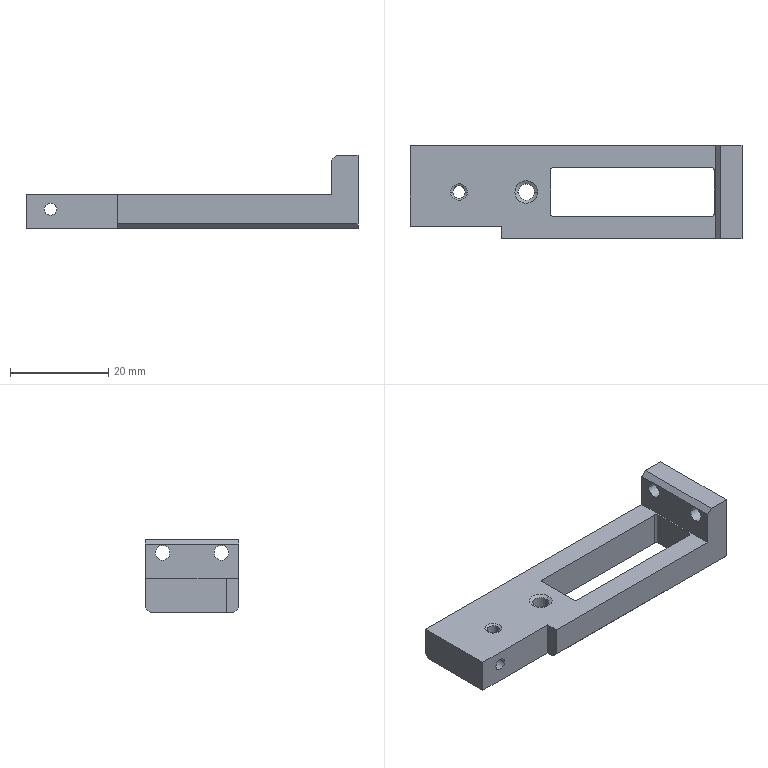Part | NX | 1 solid | 40 faces | box 67.7 x 19 x 15 mm | volume 6801 mm3 | plane 18 | cylinder 16 | cone 6 | commonest cylinder face diameters 1 x4 2.5 x4 3 x4 3.3 x2 4 x2
STEP:
#1=CARTESIAN_POINT('',(-33.85,-7.,3.5));
#2=VERTEX_POINT('',#1);
#3=CARTESIAN_POINT('',(-33.85,-7.,-3.5));
#4=VERTEX_POINT('',#3);
#5=CARTESIAN_POINT('',(-33.85,-7.,0.));
#6=DIRECTION('',(0.,0.,-1.));
#7=VECTOR('',#6,1000.);
#8=LINE('',#5,#7);
#9=EDGE_CURVE('',#2,#4,#8,.T.);
#10=ORIENTED_EDGE('',*,*,#9,.F.);
#11=CARTESIAN_POINT('',(-33.85,9.5,3.5));
#12=VERTEX_POINT('',#11);
#13=CARTESIAN_POINT('',(-33.85,0.,3.5));
#14=DIRECTION('',(0.,1.,0.));
#15=VECTOR('',#14,1000.);
#16=LINE('',#13,#15);
#17=EDGE_CURVE('',#2,#12,#16,.T.);
#18=ORIENTED_EDGE('',*,*,#17,.T.);
#19=CARTESIAN_POINT('',(-33.85,9.5,-2.5));
#20=VERTEX_POINT('',#19);
#21=CARTESIAN_POINT('',(-33.85,9.5,0.));
#22=DIRECTION('',(0.,0.,-1.));
#23=VECTOR('',#22,1000.);
#24=LINE('',#21,#23);
#25=EDGE_CURVE('',#12,#20,#24,.T.);
#26=ORIENTED_EDGE('',*,*,#25,.T.);
#27=CARTESIAN_POINT('',(-33.85,8.5,-3.5));
#28=VERTEX_POINT('',#27);
#29=CARTESIAN_POINT('',(-33.85,12.,0.));
#30=DIRECTION('',(0.,0.7071,0.7071));
#31=VECTOR('',#30,1000.);
#32=LINE('',#29,#31);
#33=EDGE_CURVE('',#28,#20,#32,.T.);
#34=ORIENTED_EDGE('',*,*,#33,.F.);
#35=CARTESIAN_POINT('',(-33.85,0.,-3.5));
#36=DIRECTION('',(0.,1.,0.));
#37=VECTOR('',#36,1000.);
#38=LINE('',#35,#37);
#39=EDGE_CURVE('',#4,#28,#38,.T.);
#40=ORIENTED_EDGE('',*,*,#39,.F.);
#41=EDGE_LOOP('',(#10,#18,#26,#34,#40));
#42=FACE_BOUND('',#41,.T.);
#43=CARTESIAN_POINT('',(-33.85,9.5,-3.5));
#44=DIRECTION('',(-1.,0.,0.));
#45=DIRECTION('',(0.,0.,1.));
#46=AXIS2_PLACEMENT_3D('',#43,#44,#45);
#47=PLANE('',#46);
#48=ADVANCED_FACE('',(#42),#47,.T.);
#49=CARTESIAN_POINT('',(-15.15,-7.,-3.5));
#50=VERTEX_POINT('',#49);
#51=CARTESIAN_POINT('',(-15.15,-8.5,-3.5));
#52=VERTEX_POINT('',#51);
#53=CARTESIAN_POINT('',(-15.15,0.,-3.5));
#54=DIRECTION('',(0.,-1.,0.));
#55=VECTOR('',#54,1000.);
#56=LINE('',#53,#55);
#57=EDGE_CURVE('',#50,#52,#56,.T.);
#58=ORIENTED_EDGE('',*,*,#57,.T.);
#59=CARTESIAN_POINT('',(-15.15,-9.5,-2.5));
#60=VERTEX_POINT('',#59);
#61=CARTESIAN_POINT('',(-15.15,-9.5,-2.5));
#62=DIRECTION('',(0.,0.7071,-0.7071));
#63=VECTOR('',#62,1000.);
#64=LINE('',#61,#63);
#65=EDGE_CURVE('',#60,#52,#64,.T.);
#66=ORIENTED_EDGE('',*,*,#65,.F.);
#67=CARTESIAN_POINT('',(-15.15,-9.5,3.5));
#68=VERTEX_POINT('',#67);
#69=CARTESIAN_POINT('',(-15.15,-9.5,3.5));
#70=DIRECTION('',(0.,0.,-1.));
#71=VECTOR('',#70,1000.);
#72=LINE('',#69,#71);
#73=EDGE_CURVE('',#68,#60,#72,.T.);
#74=ORIENTED_EDGE('',*,*,#73,.F.);
#75=CARTESIAN_POINT('',(-15.15,-7.,3.5));
#76=VERTEX_POINT('',#75);
#77=CARTESIAN_POINT('',(-15.15,0.,3.5));
#78=DIRECTION('',(0.,-1.,0.));
#79=VECTOR('',#78,1000.);
#80=LINE('',#77,#79);
#81=EDGE_CURVE('',#76,#68,#80,.T.);
#82=ORIENTED_EDGE('',*,*,#81,.F.);
#83=CARTESIAN_POINT('',(-15.15,-7.,0.));
#84=DIRECTION('',(0.,0.,1.));
#85=VECTOR('',#84,1000.);
#86=LINE('',#83,#85);
#87=EDGE_CURVE('',#50,#76,#86,.T.);
#88=ORIENTED_EDGE('',*,*,#87,.F.);
#89=EDGE_LOOP('',(#58,#66,#74,#82,#88));
#90=FACE_BOUND('',#89,.T.);
#91=CARTESIAN_POINT('',(-15.15,-9.5,3.5));
#92=DIRECTION('',(1.,0.,0.));
#93=DIRECTION('',(0.,1.,0.));
#94=AXIS2_PLACEMENT_3D('',#91,#92,#93);
#95=PLANE('',#94);
#96=ADVANCED_FACE('',(#90),#95,.F.);
#97=ORIENTED_EDGE('',*,*,#81,.T.);
#98=CARTESIAN_POINT('',(28.5,-9.5,3.5));
#99=VERTEX_POINT('',#98);
#100=CARTESIAN_POINT('',(0.,-9.5,3.5));
#101=DIRECTION('',(-1.,0.,0.));
#102=VECTOR('',#101,1000.);
#103=LINE('',#100,#102);
#104=EDGE_CURVE('',#99,#68,#103,.T.);
#105=ORIENTED_EDGE('',*,*,#104,.F.);
#106=CARTESIAN_POINT('',(28.5,9.5,3.5));
#107=VERTEX_POINT('',#106);
#108=CARTESIAN_POINT('',(28.5,0.,3.5));
#109=DIRECTION('',(0.,1.,0.));
#110=VECTOR('',#109,1000.);
#111=LINE('',#108,#110);
#112=EDGE_CURVE('',#99,#107,#111,.T.);
#113=ORIENTED_EDGE('',*,*,#112,.T.);
#114=CARTESIAN_POINT('',(0.,9.5,3.5));
#115=DIRECTION('',(1.,0.,0.));
#116=VECTOR('',#115,1000.);
#117=LINE('',#114,#116);
#118=EDGE_CURVE('',#12,#107,#117,.T.);
#119=ORIENTED_EDGE('',*,*,#118,.F.);
#120=ORIENTED_EDGE('',*,*,#17,.F.);
#121=CARTESIAN_POINT('',(0.,-7.,3.5));
#122=DIRECTION('',(1.,0.,0.));
#123=VECTOR('',#122,1000.);
#124=LINE('',#121,#123);
#125=EDGE_CURVE('',#2,#76,#124,.T.);
#126=ORIENTED_EDGE('',*,*,#125,.T.);
#127=EDGE_LOOP('',(#97,#105,#113,#119,#120,#126));
#128=FACE_BOUND('',#127,.T.);
#129=CARTESIAN_POINT('',(27.65,-5.,3.5));
#130=VERTEX_POINT('',#129);
#131=CARTESIAN_POINT('',(-4.65,-5.,3.5));
#132=VERTEX_POINT('',#131);
#133=CARTESIAN_POINT('',(0.,-5.,3.5));
#134=DIRECTION('',(-1.,0.,0.));
#135=VECTOR('',#134,1000.);
#136=LINE('',#133,#135);
#137=EDGE_CURVE('',#130,#132,#136,.T.);
#138=ORIENTED_EDGE('',*,*,#137,.T.);
#139=CARTESIAN_POINT('',(-5.15,-4.5,3.5));
#140=VERTEX_POINT('',#139);
#141=CARTESIAN_POINT('',(-4.65,-4.5,3.5));
#142=DIRECTION('',(0.,0.,1.));
#143=DIRECTION('',(0.,1.,0.));
#144=AXIS2_PLACEMENT_3D('',#141,#142,#143);
#145=CIRCLE('',#144,0.5);
#146=EDGE_CURVE('',#140,#132,#145,.T.);
#147=ORIENTED_EDGE('',*,*,#146,.F.);
#148=CARTESIAN_POINT('',(-5.15,4.5,3.5));
#149=VERTEX_POINT('',#148);
#150=CARTESIAN_POINT('',(-5.15,0.,3.5));
#151=DIRECTION('',(0.,1.,0.));
#152=VECTOR('',#151,1000.);
#153=LINE('',#150,#152);
#154=EDGE_CURVE('',#140,#149,#153,.T.);
#155=ORIENTED_EDGE('',*,*,#154,.T.);
#156=CARTESIAN_POINT('',(-4.65,5.,3.5));
#157=VERTEX_POINT('',#156);
#158=CARTESIAN_POINT('',(-4.65,4.5,3.5));
#159=DIRECTION('',(0.,0.,1.));
#160=DIRECTION('',(0.,1.,0.));
#161=AXIS2_PLACEMENT_3D('',#158,#159,#160);
#162=CIRCLE('',#161,0.5);
#163=EDGE_CURVE('',#157,#149,#162,.T.);
#164=ORIENTED_EDGE('',*,*,#163,.F.);
#165=CARTESIAN_POINT('',(27.65,5.,3.5));
#166=VERTEX_POINT('',#165);
#167=CARTESIAN_POINT('',(0.,5.,3.5));
#168=DIRECTION('',(1.,0.,0.));
#169=VECTOR('',#168,1000.);
#170=LINE('',#167,#169);
#171=EDGE_CURVE('',#157,#166,#170,.T.);
#172=ORIENTED_EDGE('',*,*,#171,.T.);
#173=CARTESIAN_POINT('',(28.15,4.5,3.5));
#174=VERTEX_POINT('',#173);
#175=CARTESIAN_POINT('',(27.65,4.5,3.5));
#176=DIRECTION('',(0.,0.,1.));
#177=DIRECTION('',(0.,1.,0.));
#178=AXIS2_PLACEMENT_3D('',#175,#176,#177);
#179=CIRCLE('',#178,0.5);
#180=EDGE_CURVE('',#174,#166,#179,.T.);
#181=ORIENTED_EDGE('',*,*,#180,.F.);
#182=CARTESIAN_POINT('',(28.15,-4.5,3.5));
#183=VERTEX_POINT('',#182);
#184=CARTESIAN_POINT('',(28.15,0.,3.5));
#185=DIRECTION('',(0.,-1.,0.));
#186=VECTOR('',#185,1000.);
#187=LINE('',#184,#186);
#188=EDGE_CURVE('',#174,#183,#187,.T.);
#189=ORIENTED_EDGE('',*,*,#188,.T.);
#190=CARTESIAN_POINT('',(27.65,-4.5,3.5));
#191=DIRECTION('',(0.,0.,1.));
#192=DIRECTION('',(0.,1.,0.));
#193=AXIS2_PLACEMENT_3D('',#190,#191,#192);
#194=CIRCLE('',#193,0.5);
#195=EDGE_CURVE('',#130,#183,#194,.T.);
#196=ORIENTED_EDGE('',*,*,#195,.F.);
#197=EDGE_LOOP('',(#138,#147,#155,#164,#172,#181,#189,#196));
#198=FACE_BOUND('',#197,.T.);
#199=CARTESIAN_POINT('',(-12.465,0.,3.5));
#200=VERTEX_POINT('',#199);
#201=CARTESIAN_POINT('',(-7.835,0.,3.5));
#202=VERTEX_POINT('',#201);
#203=CARTESIAN_POINT('',(-10.15,0.,3.5));
#204=DIRECTION('',(0.,0.,1.));
#205=DIRECTION('',(1.,0.,0.));
#206=AXIS2_PLACEMENT_3D('',#203,#204,#205);
#207=CIRCLE('',#206,2.315);
#208=EDGE_CURVE('',#200,#202,#207,.T.);
#209=ORIENTED_EDGE('',*,*,#208,.F.);
#210=CARTESIAN_POINT('',(-10.15,0.,3.5));
#211=DIRECTION('',(0.,0.,1.));
#212=DIRECTION('',(1.,0.,0.));
#213=AXIS2_PLACEMENT_3D('',#210,#211,#212);
#214=CIRCLE('',#213,2.315);
#215=EDGE_CURVE('',#202,#200,#214,.T.);
#216=ORIENTED_EDGE('',*,*,#215,.F.);
#217=EDGE_LOOP('',(#209,#216));
#218=FACE_BOUND('',#217,.T.);
#219=CARTESIAN_POINT('',(-25.55,0.,3.5));
#220=VERTEX_POINT('',#219);
#221=CARTESIAN_POINT('',(-22.15,0.,3.5));
#222=VERTEX_POINT('',#221);
#223=CARTESIAN_POINT('',(-23.85,0.,3.5));
#224=DIRECTION('',(0.,0.,1.));
#225=DIRECTION('',(1.,0.,0.));
#226=AXIS2_PLACEMENT_3D('',#223,#224,#225);
#227=CIRCLE('',#226,1.7);
#228=EDGE_CURVE('',#220,#222,#227,.T.);
#229=ORIENTED_EDGE('',*,*,#228,.F.);
#230=CARTESIAN_POINT('',(-23.85,0.,3.5));
#231=DIRECTION('',(0.,0.,1.));
#232=DIRECTION('',(1.,0.,0.));
#233=AXIS2_PLACEMENT_3D('',#230,#231,#232);
#234=CIRCLE('',#233,1.7);
#235=EDGE_CURVE('',#222,#220,#234,.T.);
#236=ORIENTED_EDGE('',*,*,#235,.F.);
#237=EDGE_LOOP('',(#229,#236));
#238=FACE_BOUND('',#237,.T.);
#239=CARTESIAN_POINT('',(0.,0.,3.5));
#240=DIRECTION('',(0.,0.,1.));
#241=DIRECTION('',(1.,0.,0.));
#242=AXIS2_PLACEMENT_3D('',#239,#240,#241);
#243=PLANE('',#242);
#244=ADVANCED_FACE('',(#128,#198,#218,#238),#243,.T.);
#245=ORIENTED_EDGE('',*,*,#112,.F.);
#246=CARTESIAN_POINT('',(28.5,-9.5,10.5));
#247=VERTEX_POINT('',#246);
#248=CARTESIAN_POINT('',(28.5,-9.5,0.));
#249=DIRECTION('',(0.,0.,-1.));
#250=VECTOR('',#249,1000.);
#251=LINE('',#248,#250);
#252=EDGE_CURVE('',#247,#99,#251,.T.);
#253=ORIENTED_EDGE('',*,*,#252,.F.);
#254=CARTESIAN_POINT('',(28.5,9.5,10.5));
#255=VERTEX_POINT('',#254);
#256=CARTESIAN_POINT('',(28.5,0.,10.5));
#257=DIRECTION('',(0.,1.,0.));
#258=VECTOR('',#257,1000.);
#259=LINE('',#256,#258);
#260=EDGE_CURVE('',#247,#255,#259,.T.);
#261=ORIENTED_EDGE('',*,*,#260,.T.);
#262=CARTESIAN_POINT('',(28.5,9.5,0.));
#263=DIRECTION('',(0.,0.,-1.));
#264=VECTOR('',#263,1000.);
#265=LINE('',#262,#264);
#266=EDGE_CURVE('',#255,#107,#265,.T.);
#267=ORIENTED_EDGE('',*,*,#266,.T.);
#268=EDGE_LOOP('',(#245,#253,#261,#267));
#269=FACE_BOUND('',#268,.T.);
#270=CARTESIAN_POINT('',(28.5,-7.5,8.73));
#271=VERTEX_POINT('',#270);
#272=CARTESIAN_POINT('',(28.5,-4.5,8.73));
#273=VERTEX_POINT('',#272);
#274=CARTESIAN_POINT('',(28.5,-6.,8.73));
#275=DIRECTION('',(1.,0.,0.));
#276=DIRECTION('',(0.,1.,0.));
#277=AXIS2_PLACEMENT_3D('',#274,#275,#276);
#278=CIRCLE('',#277,1.5);
#279=EDGE_CURVE('',#271,#273,#278,.T.);
#280=ORIENTED_EDGE('',*,*,#279,.T.);
#281=CARTESIAN_POINT('',(28.5,-6.,8.73));
#282=DIRECTION('',(1.,0.,0.));
#283=DIRECTION('',(0.,1.,0.));
#284=AXIS2_PLACEMENT_3D('',#281,#282,#283);
#285=CIRCLE('',#284,1.5);
#286=EDGE_CURVE('',#273,#271,#285,.T.);
#287=ORIENTED_EDGE('',*,*,#286,.T.);
#288=EDGE_LOOP('',(#280,#287));
#289=FACE_BOUND('',#288,.T.);
#290=CARTESIAN_POINT('',(28.5,7.5,8.73));
#291=VERTEX_POINT('',#290);
#292=CARTESIAN_POINT('',(28.5,4.5,8.73));
#293=VERTEX_POINT('',#292);
#294=CARTESIAN_POINT('',(28.5,6.,8.73));
#295=DIRECTION('',(1.,0.,0.));
#296=DIRECTION('',(0.,1.,0.));
#297=AXIS2_PLACEMENT_3D('',#294,#295,#296);
#298=CIRCLE('',#297,1.5);
#299=EDGE_CURVE('',#291,#293,#298,.T.);
#300=ORIENTED_EDGE('',*,*,#299,.T.);
#301=CARTESIAN_POINT('',(28.5,6.,8.73));
#302=DIRECTION('',(1.,0.,0.));
#303=DIRECTION('',(0.,1.,0.));
#304=AXIS2_PLACEMENT_3D('',#301,#302,#303);
#305=CIRCLE('',#304,1.5);
#306=EDGE_CURVE('',#293,#291,#305,.T.);
#307=ORIENTED_EDGE('',*,*,#306,.T.);
#308=EDGE_LOOP('',(#300,#307));
#309=FACE_BOUND('',#308,.T.);
#310=CARTESIAN_POINT('',(28.5,9.5,3.5));
#311=DIRECTION('',(-1.,0.,0.));
#312=DIRECTION('',(0.,0.,1.));
#313=AXIS2_PLACEMENT_3D('',#310,#311,#312);
#314=PLANE('',#313);
#315=ADVANCED_FACE('',(#269,#289,#309),#314,.T.);
#316=CARTESIAN_POINT('',(33.85,9.5,-2.5));
#317=VERTEX_POINT('',#316);
#318=CARTESIAN_POINT('',(0.,9.5,-2.5));
#319=DIRECTION('',(1.,0.,0.));
#320=VECTOR('',#319,1000.);
#321=LINE('',#318,#320);
#322=EDGE_CURVE('',#20,#317,#321,.T.);
#323=ORIENTED_EDGE('',*,*,#322,.F.);
#324=ORIENTED_EDGE('',*,*,#25,.F.);
#325=ORIENTED_EDGE('',*,*,#118,.T.);
#326=ORIENTED_EDGE('',*,*,#266,.F.);
#327=CARTESIAN_POINT('',(29.5,9.5,11.5));
#328=VERTEX_POINT('',#327);
#329=CARTESIAN_POINT('',(18.,9.5,0.));
#330=DIRECTION('',(0.7071,0.,0.7071));
#331=VECTOR('',#330,1000.);
#332=LINE('',#329,#331);
#333=EDGE_CURVE('',#255,#328,#332,.T.);
#334=ORIENTED_EDGE('',*,*,#333,.T.);
#335=CARTESIAN_POINT('',(33.85,9.5,11.5));
#336=VERTEX_POINT('',#335);
#337=CARTESIAN_POINT('',(0.,9.5,11.5));
#338=DIRECTION('',(-1.,0.,0.));
#339=VECTOR('',#338,1000.);
#340=LINE('',#337,#339);
#341=EDGE_CURVE('',#336,#328,#340,.T.);
#342=ORIENTED_EDGE('',*,*,#341,.F.);
#343=CARTESIAN_POINT('',(33.85,9.5,0.));
#344=DIRECTION('',(0.,0.,1.));
#345=VECTOR('',#344,1000.);
#346=LINE('',#343,#345);
#347=EDGE_CURVE('',#317,#336,#346,.T.);
#348=ORIENTED_EDGE('',*,*,#347,.F.);
#349=EDGE_LOOP('',(#323,#324,#325,#326,#334,#342,#348));
#350=FACE_BOUND('',#349,.T.);
#351=CARTESIAN_POINT('',(-30.85,9.5,0.5));
#352=VERTEX_POINT('',#351);
#353=CARTESIAN_POINT('',(-26.85,9.5,0.5));
#354=VERTEX_POINT('',#353);
#355=CARTESIAN_POINT('',(-28.85,9.5,0.5));
#356=DIRECTION('',(0.,1.,0.));
#357=DIRECTION('',(-1.,0.,0.));
#358=AXIS2_PLACEMENT_3D('',#355,#356,#357);
#359=CIRCLE('',#358,2.);
#360=EDGE_CURVE('',#352,#354,#359,.T.);
#361=ORIENTED_EDGE('',*,*,#360,.F.);
#362=CARTESIAN_POINT('',(-28.85,9.5,0.5));
#363=DIRECTION('',(0.,1.,0.));
#364=DIRECTION('',(-1.,0.,0.));
#365=AXIS2_PLACEMENT_3D('',#362,#363,#364);
#366=CIRCLE('',#365,2.);
#367=EDGE_CURVE('',#354,#352,#366,.T.);
#368=ORIENTED_EDGE('',*,*,#367,.F.);
#369=EDGE_LOOP('',(#361,#368));
#370=FACE_BOUND('',#369,.T.);
#371=CARTESIAN_POINT('',(33.85,9.5,-3.5));
#372=DIRECTION('',(0.,1.,0.));
#373=DIRECTION('',(1.,0.,0.));
#374=AXIS2_PLACEMENT_3D('',#371,#372,#373);
#375=PLANE('',#374);
#376=ADVANCED_FACE('',(#350,#370),#375,.T.);
#377=ORIENTED_EDGE('',*,*,#228,.T.);
#378=CARTESIAN_POINT('',(-22.6,0.,3.24));
#379=VERTEX_POINT('',#378);
#380=CARTESIAN_POINT('',(-22.6,0.,3.24));
#381=DIRECTION('',(0.866,0.,0.5));
#382=VECTOR('',#381,1000.);
#383=LINE('',#380,#382);
#384=EDGE_CURVE('',#379,#222,#383,.T.);
#385=ORIENTED_EDGE('',*,*,#384,.F.);
#386=CARTESIAN_POINT('',(-25.1,0.,3.24));
#387=VERTEX_POINT('',#386);
#388=CARTESIAN_POINT('',(-23.85,0.,3.24));
#389=DIRECTION('',(0.,0.,1.));
#390=DIRECTION('',(1.,0.,0.));
#391=AXIS2_PLACEMENT_3D('',#388,#389,#390);
#392=CIRCLE('',#391,1.25);
#393=EDGE_CURVE('',#387,#379,#392,.T.);
#394=ORIENTED_EDGE('',*,*,#393,.F.);
#395=CARTESIAN_POINT('',(-25.1,0.,3.24));
#396=DIRECTION('',(-0.866,0.,0.5));
#397=VECTOR('',#396,1000.);
#398=LINE('',#395,#397);
#399=EDGE_CURVE('',#387,#220,#398,.T.);
#400=ORIENTED_EDGE('',*,*,#399,.T.);
#401=EDGE_LOOP('',(#377,#385,#394,#400));
#402=FACE_BOUND('',#401,.T.);
#403=CARTESIAN_POINT('',(-23.85,0.,3.24));
#404=DIRECTION('',(0.,0.,1.));
#405=DIRECTION('',(1.,0.,0.));
#406=AXIS2_PLACEMENT_3D('',#403,#404,#405);
#407=CONICAL_SURFACE('',#406,1.25,1.047);
#408=ADVANCED_FACE('',(#402),#407,.F.);
#409=CARTESIAN_POINT('',(-25.1,0.,-3.5));
#410=VERTEX_POINT('',#409);
#411=CARTESIAN_POINT('',(-22.6,0.,-3.5));
#412=VERTEX_POINT('',#411);
#413=CARTESIAN_POINT('',(-23.85,0.,-3.5));
#414=DIRECTION('',(0.,0.,1.));
#415=DIRECTION('',(1.,0.,0.));
#416=AXIS2_PLACEMENT_3D('',#413,#414,#415);
#417=CIRCLE('',#416,1.25);
#418=EDGE_CURVE('',#410,#412,#417,.T.);
#419=ORIENTED_EDGE('',*,*,#418,.F.);
#420=CARTESIAN_POINT('',(-25.1,0.,3.5));
#421=DIRECTION('',(0.,0.,1.));
#422=VECTOR('',#421,1000.);
#423=LINE('',#420,#422);
#424=EDGE_CURVE('',#410,#387,#423,.T.);
#425=ORIENTED_EDGE('',*,*,#424,.T.);
#426=ORIENTED_EDGE('',*,*,#393,.T.);
#427=CARTESIAN_POINT('',(-22.6,0.,3.5));
#428=DIRECTION('',(0.,0.,1.));
#429=VECTOR('',#428,1000.);
#430=LINE('',#427,#429);
#431=EDGE_CURVE('',#412,#379,#430,.T.);
#432=ORIENTED_EDGE('',*,*,#431,.F.);
#433=EDGE_LOOP('',(#419,#425,#426,#432));
#434=FACE_BOUND('',#433,.T.);
#435=CARTESIAN_POINT('',(-23.85,0.,3.5));
#436=DIRECTION('',(0.,0.,1.));
#437=DIRECTION('',(1.,0.,0.));
#438=AXIS2_PLACEMENT_3D('',#435,#436,#437);
#439=CYLINDRICAL_SURFACE('',#438,1.25);
#440=ADVANCED_FACE('',(#434),#439,.F.);
#441=ORIENTED_EDGE('',*,*,#347,.T.);
#442=CARTESIAN_POINT('',(33.85,-9.5,11.5));
#443=VERTEX_POINT('',#442);
#444=CARTESIAN_POINT('',(33.85,0.,11.5));
#445=DIRECTION('',(0.,1.,0.));
#446=VECTOR('',#445,1000.);
#447=LINE('',#444,#446);
#448=EDGE_CURVE('',#443,#336,#447,.T.);
#449=ORIENTED_EDGE('',*,*,#448,.F.);
#450=CARTESIAN_POINT('',(33.85,-9.5,-2.5));
#451=VERTEX_POINT('',#450);
#452=CARTESIAN_POINT('',(33.85,-9.5,0.));
#453=DIRECTION('',(0.,0.,1.));
#454=VECTOR('',#453,1000.);
#455=LINE('',#452,#454);
#456=EDGE_CURVE('',#451,#443,#455,.T.);
#457=ORIENTED_EDGE('',*,*,#456,.F.);
#458=CARTESIAN_POINT('',(33.85,-8.5,-3.5));
#459=VERTEX_POINT('',#458);
#460=CARTESIAN_POINT('',(33.85,-12.,0.));
#461=DIRECTION('',(0.,-0.7071,0.7071));
#462=VECTOR('',#461,1000.);
#463=LINE('',#460,#462);
#464=EDGE_CURVE('',#459,#451,#463,.T.);
#465=ORIENTED_EDGE('',*,*,#464,.F.);
#466=CARTESIAN_POINT('',(33.85,8.5,-3.5));
#467=VERTEX_POINT('',#466);
#468=CARTESIAN_POINT('',(33.85,0.,-3.5));
#469=DIRECTION('',(0.,-1.,0.));
#470=VECTOR('',#469,1000.);
#471=LINE('',#468,#470);
#472=EDGE_CURVE('',#467,#459,#471,.T.);
#473=ORIENTED_EDGE('',*,*,#472,.F.);
#474=CARTESIAN_POINT('',(33.85,12.,0.));
#475=DIRECTION('',(0.,-0.7071,-0.7071));
#476=VECTOR('',#475,1000.);
#477=LINE('',#474,#476);
#478=EDGE_CURVE('',#317,#467,#477,.T.);
#479=ORIENTED_EDGE('',*,*,#478,.F.);
#480=EDGE_LOOP('',(#441,#449,#457,#465,#473,#479));
#481=FACE_BOUND('',#480,.T.);
#482=CARTESIAN_POINT('',(33.85,-4.5,8.73));
#483=VERTEX_POINT('',#482);
#484=CARTESIAN_POINT('',(33.85,-7.5,8.73));
#485=VERTEX_POINT('',#484);
#486=CARTESIAN_POINT('',(33.85,-6.,8.73));
#487=DIRECTION('',(1.,0.,0.));
#488=DIRECTION('',(0.,1.,0.));
#489=AXIS2_PLACEMENT_3D('',#486,#487,#488);
#490=CIRCLE('',#489,1.5);
#491=EDGE_CURVE('',#483,#485,#490,.T.);
#492=ORIENTED_EDGE('',*,*,#491,.F.);
#493=CARTESIAN_POINT('',(33.85,-6.,8.73));
#494=DIRECTION('',(1.,0.,0.));
#495=DIRECTION('',(0.,1.,0.));
#496=AXIS2_PLACEMENT_3D('',#493,#494,#495);
#497=CIRCLE('',#496,1.5);
#498=EDGE_CURVE('',#485,#483,#497,.T.);
#499=ORIENTED_EDGE('',*,*,#498,.F.);
#500=EDGE_LOOP('',(#492,#499));
#501=FACE_BOUND('',#500,.T.);
#502=CARTESIAN_POINT('',(33.85,7.5,8.73));
#503=VERTEX_POINT('',#502);
#504=CARTESIAN_POINT('',(33.85,4.5,8.73));
#505=VERTEX_POINT('',#504);
#506=CARTESIAN_POINT('',(33.85,6.,8.73));
#507=DIRECTION('',(1.,0.,0.));
#508=DIRECTION('',(0.,1.,0.));
#509=AXIS2_PLACEMENT_3D('',#506,#507,#508);
#510=CIRCLE('',#509,1.5);
#511=EDGE_CURVE('',#503,#505,#510,.T.);
#512=ORIENTED_EDGE('',*,*,#511,.F.);
#513=CARTESIAN_POINT('',(33.85,6.,8.73));
#514=DIRECTION('',(1.,0.,0.));
#515=DIRECTION('',(0.,1.,0.));
#516=AXIS2_PLACEMENT_3D('',#513,#514,#515);
#517=CIRCLE('',#516,1.5);
#518=EDGE_CURVE('',#505,#503,#517,.T.);
#519=ORIENTED_EDGE('',*,*,#518,.F.);
#520=EDGE_LOOP('',(#512,#519));
#521=FACE_BOUND('',#520,.T.);
#522=CARTESIAN_POINT('',(33.85,-9.5,-3.5));
#523=DIRECTION('',(1.,0.,0.));
#524=DIRECTION('',(0.,1.,0.));
#525=AXIS2_PLACEMENT_3D('',#522,#523,#524);
#526=PLANE('',#525);
#527=ADVANCED_FACE('',(#481,#501,#521),#526,.T.);
#528=ORIENTED_EDGE('',*,*,#73,.T.);
#529=CARTESIAN_POINT('',(33.85,-9.5,-2.5));
#530=DIRECTION('',(-1.,0.,0.));
#531=VECTOR('',#530,1000.);
#532=LINE('',#529,#531);
#533=EDGE_CURVE('',#451,#60,#532,.T.);
#534=ORIENTED_EDGE('',*,*,#533,.F.);
#535=ORIENTED_EDGE('',*,*,#456,.T.);
#536=CARTESIAN_POINT('',(29.5,-9.5,11.5));
#537=VERTEX_POINT('',#536);
#538=CARTESIAN_POINT('',(33.85,-9.5,11.5));
#539=DIRECTION('',(-1.,0.,0.));
#540=VECTOR('',#539,1000.);
#541=LINE('',#538,#540);
#542=EDGE_CURVE('',#443,#537,#541,.T.);
#543=ORIENTED_EDGE('',*,*,#542,.T.);
#544=CARTESIAN_POINT('',(28.5,-9.5,10.5));
#545=DIRECTION('',(0.7071,0.,0.7071));
#546=VECTOR('',#545,1000.);
#547=LINE('',#544,#546);
#548=EDGE_CURVE('',#247,#537,#547,.T.);
#549=ORIENTED_EDGE('',*,*,#548,.F.);
#550=ORIENTED_EDGE('',*,*,#252,.T.);
#551=ORIENTED_EDGE('',*,*,#104,.T.);
#552=EDGE_LOOP('',(#528,#534,#535,#543,#549,#550,#551));
#553=FACE_BOUND('',#552,.T.);
#554=CARTESIAN_POINT('',(-33.85,-9.5,-3.5));
#555=DIRECTION('',(0.,-1.,0.));
#556=DIRECTION('',(0.,0.,-1.));
#557=AXIS2_PLACEMENT_3D('',#554,#555,#556);
#558=PLANE('',#557);
#559=ADVANCED_FACE('',(#553),#558,.T.);
#560=CARTESIAN_POINT('',(0.,-7.,-3.5));
#561=DIRECTION('',(1.,0.,0.));
#562=VECTOR('',#561,1000.);
#563=LINE('',#560,#562);
#564=EDGE_CURVE('',#4,#50,#563,.T.);
#565=ORIENTED_EDGE('',*,*,#564,.T.);
#566=ORIENTED_EDGE('',*,*,#87,.T.);
#567=ORIENTED_EDGE('',*,*,#125,.F.);
#568=ORIENTED_EDGE('',*,*,#9,.T.);
#569=EDGE_LOOP('',(#565,#566,#567,#568));
#570=FACE_BOUND('',#569,.T.);
#571=CARTESIAN_POINT('',(-30.1,-7.,0.5));
#572=VERTEX_POINT('',#571);
#573=CARTESIAN_POINT('',(-27.6,-7.,0.5));
#574=VERTEX_POINT('',#573);
#575=CARTESIAN_POINT('',(-28.85,-7.,0.5));
#576=DIRECTION('',(0.,1.,0.));
#577=DIRECTION('',(1.,0.,0.));
#578=AXIS2_PLACEMENT_3D('',#575,#576,#577);
#579=CIRCLE('',#578,1.25);
#580=EDGE_CURVE('',#572,#574,#579,.T.);
#581=ORIENTED_EDGE('',*,*,#580,.T.);
#582=CARTESIAN_POINT('',(-28.85,-7.,0.5));
#583=DIRECTION('',(0.,1.,0.));
#584=DIRECTION('',(1.,0.,0.));
#585=AXIS2_PLACEMENT_3D('',#582,#583,#584);
#586=CIRCLE('',#585,1.25);
#587=EDGE_CURVE('',#574,#572,#586,.T.);
#588=ORIENTED_EDGE('',*,*,#587,.T.);
#589=EDGE_LOOP('',(#581,#588));
#590=FACE_BOUND('',#589,.T.);
#591=CARTESIAN_POINT('',(-15.15,-7.,3.5));
#592=DIRECTION('',(0.,1.,0.));
#593=DIRECTION('',(1.,0.,0.));
#594=AXIS2_PLACEMENT_3D('',#591,#592,#593);
#595=PLANE('',#594);
#596=ADVANCED_FACE('',(#570,#590),#595,.F.);
#597=CARTESIAN_POINT('',(-27.6,4.24,0.5));
#598=VERTEX_POINT('',#597);
#599=CARTESIAN_POINT('',(-30.1,4.24,0.5));
#600=VERTEX_POINT('',#599);
#601=CARTESIAN_POINT('',(-28.85,4.24,0.5));
#602=DIRECTION('',(0.,1.,0.));
#603=DIRECTION('',(1.,0.,0.));
#604=AXIS2_PLACEMENT_3D('',#601,#602,#603);
#605=CIRCLE('',#604,1.25);
#606=EDGE_CURVE('',#598,#600,#605,.T.);
#607=ORIENTED_EDGE('',*,*,#606,.F.);
#608=CARTESIAN_POINT('',(-27.15,4.5,0.5));
#609=VERTEX_POINT('',#608);
#610=CARTESIAN_POINT('',(-27.6,4.24,0.5));
#611=DIRECTION('',(0.866,0.5,0.));
#612=VECTOR('',#611,1000.);
#613=LINE('',#610,#612);
#614=EDGE_CURVE('',#598,#609,#613,.T.);
#615=ORIENTED_EDGE('',*,*,#614,.T.);
#616=CARTESIAN_POINT('',(-30.55,4.5,0.5));
#617=VERTEX_POINT('',#616);
#618=CARTESIAN_POINT('',(-28.85,4.5,0.5));
#619=DIRECTION('',(0.,1.,0.));
#620=DIRECTION('',(1.,0.,0.));
#621=AXIS2_PLACEMENT_3D('',#618,#619,#620);
#622=CIRCLE('',#621,1.7);
#623=EDGE_CURVE('',#609,#617,#622,.T.);
#624=ORIENTED_EDGE('',*,*,#623,.T.);
#625=CARTESIAN_POINT('',(-30.1,4.24,0.5));
#626=DIRECTION('',(-0.866,0.5,0.));
#627=VECTOR('',#626,1000.);
#628=LINE('',#625,#627);
#629=EDGE_CURVE('',#600,#617,#628,.T.);
#630=ORIENTED_EDGE('',*,*,#629,.F.);
#631=EDGE_LOOP('',(#607,#615,#624,#630));
#632=FACE_BOUND('',#631,.T.);
#633=CARTESIAN_POINT('',(-28.85,4.24,0.5));
#634=DIRECTION('',(0.,1.,0.));
#635=DIRECTION('',(1.,0.,0.));
#636=AXIS2_PLACEMENT_3D('',#633,#634,#635);
#637=CONICAL_SURFACE('',#636,1.25,1.047);
#638=ADVANCED_FACE('',(#632),#637,.F.);
#639=ORIENTED_EDGE('',*,*,#448,.T.);
#640=ORIENTED_EDGE('',*,*,#341,.T.);
#641=CARTESIAN_POINT('',(29.5,-9.5,11.5));
#642=DIRECTION('',(0.,1.,0.));
#643=VECTOR('',#642,1000.);
#644=LINE('',#641,#643);
#645=EDGE_CURVE('',#537,#328,#644,.T.);
#646=ORIENTED_EDGE('',*,*,#645,.F.);
#647=ORIENTED_EDGE('',*,*,#542,.F.);
#648=EDGE_LOOP('',(#639,#640,#646,#647));
#649=FACE_BOUND('',#648,.T.);
#650=CARTESIAN_POINT('',(0.,0.,11.5));
#651=DIRECTION('',(0.,0.,1.));
#652=DIRECTION('',(1.,0.,0.));
#653=AXIS2_PLACEMENT_3D('',#650,#651,#652);
#654=PLANE('',#653);
#655=ADVANCED_FACE('',(#649),#654,.T.);
#656=ORIENTED_EDGE('',*,*,#645,.T.);
#657=ORIENTED_EDGE('',*,*,#333,.F.);
#658=ORIENTED_EDGE('',*,*,#260,.F.);
#659=ORIENTED_EDGE('',*,*,#548,.T.);
#660=EDGE_LOOP('',(#656,#657,#658,#659));
#661=FACE_BOUND('',#660,.T.);
#662=CARTESIAN_POINT('',(29.5,9.5,11.5));
#663=DIRECTION('',(0.7071,0.,-0.7071));
#664=DIRECTION('',(0.,-1.,0.));
#665=AXIS2_PLACEMENT_3D('',#662,#663,#664);
#666=PLANE('',#665);
#667=ADVANCED_FACE('',(#661),#666,.F.);
#668=CARTESIAN_POINT('',(0.,8.5,-3.5));
#669=DIRECTION('',(1.,0.,0.));
#670=VECTOR('',#669,1000.);
#671=LINE('',#668,#670);
#672=EDGE_CURVE('',#28,#467,#671,.T.);
#673=ORIENTED_EDGE('',*,*,#672,.T.);
#674=ORIENTED_EDGE('',*,*,#472,.T.);
#675=CARTESIAN_POINT('',(0.,-8.5,-3.5));
#676=DIRECTION('',(-1.,0.,0.));
#677=VECTOR('',#676,1000.);
#678=LINE('',#675,#677);
#679=EDGE_CURVE('',#459,#52,#678,.T.);
#680=ORIENTED_EDGE('',*,*,#679,.T.);
#681=ORIENTED_EDGE('',*,*,#57,.F.);
#682=ORIENTED_EDGE('',*,*,#564,.F.);
#683=ORIENTED_EDGE('',*,*,#39,.T.);
#684=EDGE_LOOP('',(#673,#674,#680,#681,#682,#683));
#685=FACE_BOUND('',#684,.T.);
#686=CARTESIAN_POINT('',(27.65,-5.,-3.5));
#687=VERTEX_POINT('',#686);
#688=CARTESIAN_POINT('',(-4.65,-5.,-3.5));
#689=VERTEX_POINT('',#688);
#690=CARTESIAN_POINT('',(0.,-5.,-3.5));
#691=DIRECTION('',(-1.,0.,0.));
#692=VECTOR('',#691,1000.);
#693=LINE('',#690,#692);
#694=EDGE_CURVE('',#687,#689,#693,.T.);
#695=ORIENTED_EDGE('',*,*,#694,.F.);
#696=CARTESIAN_POINT('',(28.15,-4.5,-3.5));
#697=VERTEX_POINT('',#696);
#698=CARTESIAN_POINT('',(27.65,-4.5,-3.5));
#699=DIRECTION('',(0.,0.,1.));
#700=DIRECTION('',(0.,1.,0.));
#701=AXIS2_PLACEMENT_3D('',#698,#699,#700);
#702=CIRCLE('',#701,0.5);
#703=EDGE_CURVE('',#687,#697,#702,.T.);
#704=ORIENTED_EDGE('',*,*,#703,.T.);
#705=CARTESIAN_POINT('',(28.15,4.5,-3.5));
#706=VERTEX_POINT('',#705);
#707=CARTESIAN_POINT('',(28.15,0.,-3.5));
#708=DIRECTION('',(0.,-1.,0.));
#709=VECTOR('',#708,1000.);
#710=LINE('',#707,#709);
#711=EDGE_CURVE('',#706,#697,#710,.T.);
#712=ORIENTED_EDGE('',*,*,#711,.F.);
#713=CARTESIAN_POINT('',(27.65,5.,-3.5));
#714=VERTEX_POINT('',#713);
#715=CARTESIAN_POINT('',(27.65,4.5,-3.5));
#716=DIRECTION('',(0.,0.,1.));
#717=DIRECTION('',(0.,1.,0.));
#718=AXIS2_PLACEMENT_3D('',#715,#716,#717);
#719=CIRCLE('',#718,0.5);
#720=EDGE_CURVE('',#706,#714,#719,.T.);
#721=ORIENTED_EDGE('',*,*,#720,.T.);
#722=CARTESIAN_POINT('',(-4.65,5.,-3.5));
#723=VERTEX_POINT('',#722);
#724=CARTESIAN_POINT('',(0.,5.,-3.5));
#725=DIRECTION('',(1.,0.,0.));
#726=VECTOR('',#725,1000.);
#727=LINE('',#724,#726);
#728=EDGE_CURVE('',#723,#714,#727,.T.);
#729=ORIENTED_EDGE('',*,*,#728,.F.);
#730=CARTESIAN_POINT('',(-5.15,4.5,-3.5));
#731=VERTEX_POINT('',#730);
#732=CARTESIAN_POINT('',(-4.65,4.5,-3.5));
#733=DIRECTION('',(0.,0.,1.));
#734=DIRECTION('',(0.,1.,0.));
#735=AXIS2_PLACEMENT_3D('',#732,#733,#734);
#736=CIRCLE('',#735,0.5);
#737=EDGE_CURVE('',#723,#731,#736,.T.);
#738=ORIENTED_EDGE('',*,*,#737,.T.);
#739=CARTESIAN_POINT('',(-5.15,-4.5,-3.5));
#740=VERTEX_POINT('',#739);
#741=CARTESIAN_POINT('',(-5.15,0.,-3.5));
#742=DIRECTION('',(0.,1.,0.));
#743=VECTOR('',#742,1000.);
#744=LINE('',#741,#743);
#745=EDGE_CURVE('',#740,#731,#744,.T.);
#746=ORIENTED_EDGE('',*,*,#745,.F.);
#747=CARTESIAN_POINT('',(-4.65,-4.5,-3.5));
#748=DIRECTION('',(0.,0.,1.));
#749=DIRECTION('',(0.,1.,0.));
#750=AXIS2_PLACEMENT_3D('',#747,#748,#749);
#751=CIRCLE('',#750,0.5);
#752=EDGE_CURVE('',#740,#689,#751,.T.);
#753=ORIENTED_EDGE('',*,*,#752,.T.);
#754=EDGE_LOOP('',(#695,#704,#712,#721,#729,#738,#746,#753));
#755=FACE_BOUND('',#754,.T.);
#756=ORIENTED_EDGE('',*,*,#418,.T.);
#757=CARTESIAN_POINT('',(-23.85,0.,-3.5));
#758=DIRECTION('',(0.,0.,1.));
#759=DIRECTION('',(1.,0.,0.));
#760=AXIS2_PLACEMENT_3D('',#757,#758,#759);
#761=CIRCLE('',#760,1.25);
#762=EDGE_CURVE('',#412,#410,#761,.T.);
#763=ORIENTED_EDGE('',*,*,#762,.T.);
#764=EDGE_LOOP('',(#756,#763));
#765=FACE_BOUND('',#764,.T.);
#766=CARTESIAN_POINT('',(-8.5,0.,-3.5));
#767=VERTEX_POINT('',#766);
#768=CARTESIAN_POINT('',(-11.8,0.,-3.5));
#769=VERTEX_POINT('',#768);
#770=CARTESIAN_POINT('',(-10.15,0.,-3.5));
#771=DIRECTION('',(0.,0.,1.));
#772=DIRECTION('',(1.,0.,0.));
#773=AXIS2_PLACEMENT_3D('',#770,#771,#772);
#774=CIRCLE('',#773,1.65);
#775=EDGE_CURVE('',#767,#769,#774,.T.);
#776=ORIENTED_EDGE('',*,*,#775,.T.);
#777=CARTESIAN_POINT('',(-10.15,0.,-3.5));
#778=DIRECTION('',(0.,0.,1.));
#779=DIRECTION('',(1.,0.,0.));
#780=AXIS2_PLACEMENT_3D('',#777,#778,#779);
#781=CIRCLE('',#780,1.65);
#782=EDGE_CURVE('',#769,#767,#781,.T.);
#783=ORIENTED_EDGE('',*,*,#782,.T.);
#784=EDGE_LOOP('',(#776,#783));
#785=FACE_BOUND('',#784,.T.);
#786=CARTESIAN_POINT('',(0.,0.,-3.5));
#787=DIRECTION('',(0.,0.,1.));
#788=DIRECTION('',(1.,0.,0.));
#789=AXIS2_PLACEMENT_3D('',#786,#787,#788);
#790=PLANE('',#789);
#791=ADVANCED_FACE('',(#685,#755,#765,#785),#790,.F.);
#792=ORIENTED_EDGE('',*,*,#279,.F.);
#793=CARTESIAN_POINT('',(28.5,-7.5,8.73));
#794=DIRECTION('',(1.,0.,0.));
#795=VECTOR('',#794,1000.);
#796=LINE('',#793,#795);
#797=EDGE_CURVE('',#485,#271,#796,.F.);
#798=ORIENTED_EDGE('',*,*,#797,.F.);
#799=ORIENTED_EDGE('',*,*,#498,.T.);
#800=CARTESIAN_POINT('',(28.5,-4.5,8.73));
#801=DIRECTION('',(1.,0.,0.));
#802=VECTOR('',#801,1000.);
#803=LINE('',#800,#802);
#804=EDGE_CURVE('',#483,#273,#803,.F.);
#805=ORIENTED_EDGE('',*,*,#804,.T.);
#806=EDGE_LOOP('',(#792,#798,#799,#805));
#807=FACE_BOUND('',#806,.T.);
#808=CARTESIAN_POINT('',(28.5,-6.,8.73));
#809=DIRECTION('',(1.,0.,0.));
#810=DIRECTION('',(0.,1.,0.));
#811=AXIS2_PLACEMENT_3D('',#808,#809,#810);
#812=CYLINDRICAL_SURFACE('',#811,1.5);
#813=ADVANCED_FACE('',(#807),#812,.F.);
#814=ORIENTED_EDGE('',*,*,#679,.F.);
#815=ORIENTED_EDGE('',*,*,#464,.T.);
#816=ORIENTED_EDGE('',*,*,#533,.T.);
#817=ORIENTED_EDGE('',*,*,#65,.T.);
#818=EDGE_LOOP('',(#814,#815,#816,#817));
#819=FACE_BOUND('',#818,.T.);
#820=CARTESIAN_POINT('',(-15.15,-8.5,-3.5));
#821=DIRECTION('',(0.,-0.7071,-0.7071));
#822=DIRECTION('',(0.,-0.7071,0.7071));
#823=AXIS2_PLACEMENT_3D('',#820,#821,#822);
#824=PLANE('',#823);
#825=ADVANCED_FACE('',(#819),#824,.T.);
#826=ORIENTED_EDGE('',*,*,#511,.T.);
#827=CARTESIAN_POINT('',(28.5,4.5,8.73));
#828=DIRECTION('',(1.,0.,0.));
#829=VECTOR('',#828,1000.);
#830=LINE('',#827,#829);
#831=EDGE_CURVE('',#293,#505,#830,.T.);
#832=ORIENTED_EDGE('',*,*,#831,.F.);
#833=ORIENTED_EDGE('',*,*,#299,.F.);
#834=CARTESIAN_POINT('',(28.5,7.5,8.73));
#835=DIRECTION('',(1.,0.,0.));
#836=VECTOR('',#835,1000.);
#837=LINE('',#834,#836);
#838=EDGE_CURVE('',#291,#503,#837,.T.);
#839=ORIENTED_EDGE('',*,*,#838,.T.);
#840=EDGE_LOOP('',(#826,#832,#833,#839));
#841=FACE_BOUND('',#840,.T.);
#842=CARTESIAN_POINT('',(28.5,6.,8.73));
#843=DIRECTION('',(1.,0.,0.));
#844=DIRECTION('',(0.,1.,0.));
#845=AXIS2_PLACEMENT_3D('',#842,#843,#844);
#846=CYLINDRICAL_SURFACE('',#845,1.5);
#847=ADVANCED_FACE('',(#841),#846,.F.);
#848=ORIENTED_EDGE('',*,*,#580,.F.);
#849=CARTESIAN_POINT('',(-30.1,4.5,0.5));
#850=DIRECTION('',(0.,1.,0.));
#851=VECTOR('',#850,1000.);
#852=LINE('',#849,#851);
#853=EDGE_CURVE('',#600,#572,#852,.F.);
#854=ORIENTED_EDGE('',*,*,#853,.F.);
#855=CARTESIAN_POINT('',(-28.85,4.24,0.5));
#856=DIRECTION('',(0.,1.,0.));
#857=DIRECTION('',(1.,0.,0.));
#858=AXIS2_PLACEMENT_3D('',#855,#856,#857);
#859=CIRCLE('',#858,1.25);
#860=EDGE_CURVE('',#600,#598,#859,.T.);
#861=ORIENTED_EDGE('',*,*,#860,.T.);
#862=CARTESIAN_POINT('',(-27.6,4.5,0.5));
#863=DIRECTION('',(0.,1.,0.));
#864=VECTOR('',#863,1000.);
#865=LINE('',#862,#864);
#866=EDGE_CURVE('',#598,#574,#865,.F.);
#867=ORIENTED_EDGE('',*,*,#866,.T.);
#868=EDGE_LOOP('',(#848,#854,#861,#867));
#869=FACE_BOUND('',#868,.T.);
#870=CARTESIAN_POINT('',(-28.85,4.5,0.5));
#871=DIRECTION('',(0.,1.,0.));
#872=DIRECTION('',(1.,0.,0.));
#873=AXIS2_PLACEMENT_3D('',#870,#871,#872);
#874=CYLINDRICAL_SURFACE('',#873,1.25);
#875=ADVANCED_FACE('',(#869),#874,.F.);
#876=ORIENTED_EDGE('',*,*,#694,.T.);
#877=CARTESIAN_POINT('',(-4.65,-5.,3.5));
#878=DIRECTION('',(0.,0.,1.));
#879=VECTOR('',#878,1000.);
#880=LINE('',#877,#879);
#881=EDGE_CURVE('',#689,#132,#880,.T.);
#882=ORIENTED_EDGE('',*,*,#881,.T.);
#883=ORIENTED_EDGE('',*,*,#137,.F.);
#884=CARTESIAN_POINT('',(27.65,-5.,3.5));
#885=DIRECTION('',(0.,0.,1.));
#886=VECTOR('',#885,1000.);
#887=LINE('',#884,#886);
#888=EDGE_CURVE('',#687,#130,#887,.T.);
#889=ORIENTED_EDGE('',*,*,#888,.F.);
#890=EDGE_LOOP('',(#876,#882,#883,#889));
#891=FACE_BOUND('',#890,.T.);
#892=CARTESIAN_POINT('',(-4.65,-5.,3.5));
#893=DIRECTION('',(0.,-1.,0.));
#894=DIRECTION('',(0.,0.,-1.));
#895=AXIS2_PLACEMENT_3D('',#892,#893,#894);
#896=PLANE('',#895);
#897=ADVANCED_FACE('',(#891),#896,.F.);
#898=ORIENTED_EDGE('',*,*,#703,.F.);
#899=ORIENTED_EDGE('',*,*,#888,.T.);
#900=ORIENTED_EDGE('',*,*,#195,.T.);
#901=CARTESIAN_POINT('',(28.15,-4.5,-3.5));
#902=DIRECTION('',(0.,0.,1.));
#903=VECTOR('',#902,1000.);
#904=LINE('',#901,#903);
#905=EDGE_CURVE('',#697,#183,#904,.T.);
#906=ORIENTED_EDGE('',*,*,#905,.F.);
#907=EDGE_LOOP('',(#898,#899,#900,#906));
#908=FACE_BOUND('',#907,.T.);
#909=CARTESIAN_POINT('',(27.65,-4.5,3.5));
#910=DIRECTION('',(0.,0.,1.));
#911=DIRECTION('',(0.,1.,0.));
#912=AXIS2_PLACEMENT_3D('',#909,#910,#911);
#913=CYLINDRICAL_SURFACE('',#912,0.5);
#914=ADVANCED_FACE('',(#908),#913,.F.);
#915=ORIENTED_EDGE('',*,*,#711,.T.);
#916=ORIENTED_EDGE('',*,*,#905,.T.);
#917=ORIENTED_EDGE('',*,*,#188,.F.);
#918=CARTESIAN_POINT('',(28.15,4.5,3.5));
#919=DIRECTION('',(0.,0.,-1.));
#920=VECTOR('',#919,1000.);
#921=LINE('',#918,#920);
#922=EDGE_CURVE('',#174,#706,#921,.T.);
#923=ORIENTED_EDGE('',*,*,#922,.T.);
#924=EDGE_LOOP('',(#915,#916,#917,#923));
#925=FACE_BOUND('',#924,.T.);
#926=CARTESIAN_POINT('',(28.15,-4.5,3.5));
#927=DIRECTION('',(1.,0.,0.));
#928=DIRECTION('',(0.,1.,0.));
#929=AXIS2_PLACEMENT_3D('',#926,#927,#928);
#930=PLANE('',#929);
#931=ADVANCED_FACE('',(#925),#930,.F.);
#932=ORIENTED_EDGE('',*,*,#720,.F.);
#933=ORIENTED_EDGE('',*,*,#922,.F.);
#934=ORIENTED_EDGE('',*,*,#180,.T.);
#935=CARTESIAN_POINT('',(27.65,5.,3.5));
#936=DIRECTION('',(0.,0.,1.));
#937=VECTOR('',#936,1000.);
#938=LINE('',#935,#937);
#939=EDGE_CURVE('',#714,#166,#938,.T.);
#940=ORIENTED_EDGE('',*,*,#939,.F.);
#941=EDGE_LOOP('',(#932,#933,#934,#940));
#942=FACE_BOUND('',#941,.T.);
#943=CARTESIAN_POINT('',(27.65,4.5,3.5));
#944=DIRECTION('',(0.,0.,1.));
#945=DIRECTION('',(0.,1.,0.));
#946=AXIS2_PLACEMENT_3D('',#943,#944,#945);
#947=CYLINDRICAL_SURFACE('',#946,0.5);
#948=ADVANCED_FACE('',(#942),#947,.F.);
#949=ORIENTED_EDGE('',*,*,#728,.T.);
#950=ORIENTED_EDGE('',*,*,#939,.T.);
#951=ORIENTED_EDGE('',*,*,#171,.F.);
#952=CARTESIAN_POINT('',(-4.65,5.,3.5));
#953=DIRECTION('',(0.,0.,1.));
#954=VECTOR('',#953,1000.);
#955=LINE('',#952,#954);
#956=EDGE_CURVE('',#723,#157,#955,.T.);
#957=ORIENTED_EDGE('',*,*,#956,.F.);
#958=EDGE_LOOP('',(#949,#950,#951,#957));
#959=FACE_BOUND('',#958,.T.);
#960=CARTESIAN_POINT('',(27.65,5.,3.5));
#961=DIRECTION('',(0.,1.,0.));
#962=DIRECTION('',(1.,0.,0.));
#963=AXIS2_PLACEMENT_3D('',#960,#961,#962);
#964=PLANE('',#963);
#965=ADVANCED_FACE('',(#959),#964,.F.);
#966=ORIENTED_EDGE('',*,*,#737,.F.);
#967=ORIENTED_EDGE('',*,*,#956,.T.);
#968=ORIENTED_EDGE('',*,*,#163,.T.);
#969=CARTESIAN_POINT('',(-5.15,4.5,-3.5));
#970=DIRECTION('',(0.,0.,1.));
#971=VECTOR('',#970,1000.);
#972=LINE('',#969,#971);
#973=EDGE_CURVE('',#731,#149,#972,.T.);
#974=ORIENTED_EDGE('',*,*,#973,.F.);
#975=EDGE_LOOP('',(#966,#967,#968,#974));
#976=FACE_BOUND('',#975,.T.);
#977=CARTESIAN_POINT('',(-4.65,4.5,3.5));
#978=DIRECTION('',(0.,0.,1.));
#979=DIRECTION('',(0.,1.,0.));
#980=AXIS2_PLACEMENT_3D('',#977,#978,#979);
#981=CYLINDRICAL_SURFACE('',#980,0.5);
#982=ADVANCED_FACE('',(#976),#981,.F.);
#983=ORIENTED_EDGE('',*,*,#745,.T.);
#984=ORIENTED_EDGE('',*,*,#973,.T.);
#985=ORIENTED_EDGE('',*,*,#154,.F.);
#986=CARTESIAN_POINT('',(-5.15,-4.5,3.5));
#987=DIRECTION('',(0.,0.,-1.));
#988=VECTOR('',#987,1000.);
#989=LINE('',#986,#988);
#990=EDGE_CURVE('',#140,#740,#989,.T.);
#991=ORIENTED_EDGE('',*,*,#990,.T.);
#992=EDGE_LOOP('',(#983,#984,#985,#991));
#993=FACE_BOUND('',#992,.T.);
#994=CARTESIAN_POINT('',(-5.15,4.5,3.5));
#995=DIRECTION('',(-1.,0.,0.));
#996=DIRECTION('',(0.,0.,1.));
#997=AXIS2_PLACEMENT_3D('',#994,#995,#996);
#998=PLANE('',#997);
#999=ADVANCED_FACE('',(#993),#998,.F.);
#1000=ORIENTED_EDGE('',*,*,#752,.F.);
#1001=ORIENTED_EDGE('',*,*,#990,.F.);
#1002=ORIENTED_EDGE('',*,*,#146,.T.);
#1003=ORIENTED_EDGE('',*,*,#881,.F.);
#1004=EDGE_LOOP('',(#1000,#1001,#1002,#1003));
#1005=FACE_BOUND('',#1004,.T.);
#1006=CARTESIAN_POINT('',(-4.65,-4.5,3.5));
#1007=DIRECTION('',(0.,0.,1.));
#1008=DIRECTION('',(0.,1.,0.));
#1009=AXIS2_PLACEMENT_3D('',#1006,#1007,#1008);
#1010=CYLINDRICAL_SURFACE('',#1009,0.5);
#1011=ADVANCED_FACE('',(#1005),#1010,.F.);
#1012=ORIENTED_EDGE('',*,*,#672,.F.);
#1013=ORIENTED_EDGE('',*,*,#33,.T.);
#1014=ORIENTED_EDGE('',*,*,#322,.T.);
#1015=ORIENTED_EDGE('',*,*,#478,.T.);
#1016=EDGE_LOOP('',(#1012,#1013,#1014,#1015));
#1017=FACE_BOUND('',#1016,.T.);
#1018=CARTESIAN_POINT('',(0.,9.,-3.));
#1019=DIRECTION('',(0.,0.7071,-0.7071));
#1020=DIRECTION('',(-1.,0.,0.));
#1021=AXIS2_PLACEMENT_3D('',#1018,#1019,#1020);
#1022=PLANE('',#1021);
#1023=ADVANCED_FACE('',(#1017),#1022,.T.);
#1024=CARTESIAN_POINT('',(-26.85,4.5,0.5));
#1025=VERTEX_POINT('',#1024);
#1026=CARTESIAN_POINT('',(-30.85,4.5,0.5));
#1027=VERTEX_POINT('',#1026);
#1028=CARTESIAN_POINT('',(-28.85,4.5,0.5));
#1029=DIRECTION('',(0.,1.,0.));
#1030=DIRECTION('',(-1.,0.,0.));
#1031=AXIS2_PLACEMENT_3D('',#1028,#1029,#1030);
#1032=CIRCLE('',#1031,2.);
#1033=EDGE_CURVE('',#1025,#1027,#1032,.T.);
#1034=ORIENTED_EDGE('',*,*,#1033,.F.);
#1035=CARTESIAN_POINT('',(-26.85,9.5,0.5));
#1036=DIRECTION('',(0.,1.,0.));
#1037=VECTOR('',#1036,1000.);
#1038=LINE('',#1035,#1037);
#1039=EDGE_CURVE('',#1025,#354,#1038,.T.);
#1040=ORIENTED_EDGE('',*,*,#1039,.T.);
#1041=ORIENTED_EDGE('',*,*,#367,.T.);
#1042=CARTESIAN_POINT('',(-30.85,9.5,0.5));
#1043=DIRECTION('',(0.,1.,0.));
#1044=VECTOR('',#1043,1000.);
#1045=LINE('',#1042,#1044);
#1046=EDGE_CURVE('',#1027,#352,#1045,.T.);
#1047=ORIENTED_EDGE('',*,*,#1046,.F.);
#1048=EDGE_LOOP('',(#1034,#1040,#1041,#1047));
#1049=FACE_BOUND('',#1048,.T.);
#1050=CARTESIAN_POINT('',(-28.85,9.5,0.5));
#1051=DIRECTION('',(0.,1.,0.));
#1052=DIRECTION('',(-1.,0.,0.));
#1053=AXIS2_PLACEMENT_3D('',#1050,#1051,#1052);
#1054=CYLINDRICAL_SURFACE('',#1053,2.);
#1055=ADVANCED_FACE('',(#1049),#1054,.F.);
#1056=ORIENTED_EDGE('',*,*,#1033,.T.);
#1057=CARTESIAN_POINT('',(-28.85,4.5,0.5));
#1058=DIRECTION('',(0.,1.,0.));
#1059=DIRECTION('',(-1.,0.,0.));
#1060=AXIS2_PLACEMENT_3D('',#1057,#1058,#1059);
#1061=CIRCLE('',#1060,2.);
#1062=EDGE_CURVE('',#1027,#1025,#1061,.T.);
#1063=ORIENTED_EDGE('',*,*,#1062,.T.);
#1064=EDGE_LOOP('',(#1056,#1063));
#1065=FACE_BOUND('',#1064,.T.);
#1066=ORIENTED_EDGE('',*,*,#623,.F.);
#1067=CARTESIAN_POINT('',(-28.85,4.5,0.5));
#1068=DIRECTION('',(0.,1.,0.));
#1069=DIRECTION('',(1.,0.,0.));
#1070=AXIS2_PLACEMENT_3D('',#1067,#1068,#1069);
#1071=CIRCLE('',#1070,1.7);
#1072=EDGE_CURVE('',#617,#609,#1071,.T.);
#1073=ORIENTED_EDGE('',*,*,#1072,.F.);
#1074=EDGE_LOOP('',(#1066,#1073));
#1075=FACE_BOUND('',#1074,.T.);
#1076=CARTESIAN_POINT('',(-31.585,4.5,-1.286));
#1077=DIRECTION('',(0.,1.,0.));
#1078=DIRECTION('',(1.,0.,0.));
#1079=AXIS2_PLACEMENT_3D('',#1076,#1077,#1078);
#1080=PLANE('',#1079);
#1081=ADVANCED_FACE('',(#1065,#1075),#1080,.T.);
#1082=CARTESIAN_POINT('',(-11.8,0.,3.116));
#1083=VERTEX_POINT('',#1082);
#1084=CARTESIAN_POINT('',(-8.5,0.,3.116));
#1085=VERTEX_POINT('',#1084);
#1086=CARTESIAN_POINT('',(-10.15,0.,3.116));
#1087=DIRECTION('',(0.,0.,1.));
#1088=DIRECTION('',(1.,0.,0.));
#1089=AXIS2_PLACEMENT_3D('',#1086,#1087,#1088);
#1090=CIRCLE('',#1089,1.65);
#1091=EDGE_CURVE('',#1083,#1085,#1090,.T.);
#1092=ORIENTED_EDGE('',*,*,#1091,.T.);
#1093=CARTESIAN_POINT('',(-8.5,0.,3.5));
#1094=DIRECTION('',(0.,0.,1.));
#1095=VECTOR('',#1094,1000.);
#1096=LINE('',#1093,#1095);
#1097=EDGE_CURVE('',#767,#1085,#1096,.T.);
#1098=ORIENTED_EDGE('',*,*,#1097,.F.);
#1099=ORIENTED_EDGE('',*,*,#782,.F.);
#1100=CARTESIAN_POINT('',(-11.8,0.,3.5));
#1101=DIRECTION('',(0.,0.,1.));
#1102=VECTOR('',#1101,1000.);
#1103=LINE('',#1100,#1102);
#1104=EDGE_CURVE('',#769,#1083,#1103,.T.);
#1105=ORIENTED_EDGE('',*,*,#1104,.T.);
#1106=EDGE_LOOP('',(#1092,#1098,#1099,#1105));
#1107=FACE_BOUND('',#1106,.T.);
#1108=CARTESIAN_POINT('',(-10.15,0.,3.5));
#1109=DIRECTION('',(0.,0.,1.));
#1110=DIRECTION('',(1.,0.,0.));
#1111=AXIS2_PLACEMENT_3D('',#1108,#1109,#1110);
#1112=CYLINDRICAL_SURFACE('',#1111,1.65);
#1113=ADVANCED_FACE('',(#1107),#1112,.F.);
#1114=ORIENTED_EDGE('',*,*,#208,.T.);
#1115=CARTESIAN_POINT('',(-8.5,0.,3.116));
#1116=DIRECTION('',(0.866,0.,0.5));
#1117=VECTOR('',#1116,1000.);
#1118=LINE('',#1115,#1117);
#1119=EDGE_CURVE('',#1085,#202,#1118,.T.);
#1120=ORIENTED_EDGE('',*,*,#1119,.F.);
#1121=ORIENTED_EDGE('',*,*,#1091,.F.);
#1122=CARTESIAN_POINT('',(-11.8,0.,3.116));
#1123=DIRECTION('',(-0.866,0.,0.5));
#1124=VECTOR('',#1123,1000.);
#1125=LINE('',#1122,#1124);
#1126=EDGE_CURVE('',#1083,#200,#1125,.T.);
#1127=ORIENTED_EDGE('',*,*,#1126,.T.);
#1128=EDGE_LOOP('',(#1114,#1120,#1121,#1127));
#1129=FACE_BOUND('',#1128,.T.);
#1130=CARTESIAN_POINT('',(-10.15,0.,3.116));
#1131=DIRECTION('',(0.,0.,1.));
#1132=DIRECTION('',(1.,0.,0.));
#1133=AXIS2_PLACEMENT_3D('',#1130,#1131,#1132);
#1134=CONICAL_SURFACE('',#1133,1.65,1.047);
#1135=ADVANCED_FACE('',(#1129),#1134,.F.);
#1136=ORIENTED_EDGE('',*,*,#1119,.T.);
#1137=ORIENTED_EDGE('',*,*,#215,.T.);
#1138=ORIENTED_EDGE('',*,*,#1126,.F.);
#1139=CARTESIAN_POINT('',(-10.15,0.,3.116));
#1140=DIRECTION('',(0.,0.,1.));
#1141=DIRECTION('',(1.,0.,0.));
#1142=AXIS2_PLACEMENT_3D('',#1139,#1140,#1141);
#1143=CIRCLE('',#1142,1.65);
#1144=EDGE_CURVE('',#1085,#1083,#1143,.T.);
#1145=ORIENTED_EDGE('',*,*,#1144,.F.);
#1146=EDGE_LOOP('',(#1136,#1137,#1138,#1145));
#1147=FACE_BOUND('',#1146,.T.);
#1148=CARTESIAN_POINT('',(-10.15,0.,3.116));
#1149=DIRECTION('',(0.,0.,1.));
#1150=DIRECTION('',(1.,0.,0.));
#1151=AXIS2_PLACEMENT_3D('',#1148,#1149,#1150);
#1152=CONICAL_SURFACE('',#1151,1.65,1.047);
#1153=ADVANCED_FACE('',(#1147),#1152,.F.);
#1154=ORIENTED_EDGE('',*,*,#431,.T.);
#1155=CARTESIAN_POINT('',(-23.85,0.,3.24));
#1156=DIRECTION('',(0.,0.,1.));
#1157=DIRECTION('',(1.,0.,0.));
#1158=AXIS2_PLACEMENT_3D('',#1155,#1156,#1157);
#1159=CIRCLE('',#1158,1.25);
#1160=EDGE_CURVE('',#379,#387,#1159,.T.);
#1161=ORIENTED_EDGE('',*,*,#1160,.T.);
#1162=ORIENTED_EDGE('',*,*,#424,.F.);
#1163=ORIENTED_EDGE('',*,*,#762,.F.);
#1164=EDGE_LOOP('',(#1154,#1161,#1162,#1163));
#1165=FACE_BOUND('',#1164,.T.);
#1166=CARTESIAN_POINT('',(-23.85,0.,3.5));
#1167=DIRECTION('',(0.,0.,1.));
#1168=DIRECTION('',(1.,0.,0.));
#1169=AXIS2_PLACEMENT_3D('',#1166,#1167,#1168);
#1170=CYLINDRICAL_SURFACE('',#1169,1.25);
#1171=ADVANCED_FACE('',(#1165),#1170,.F.);
#1172=ORIENTED_EDGE('',*,*,#838,.F.);
#1173=ORIENTED_EDGE('',*,*,#306,.F.);
#1174=ORIENTED_EDGE('',*,*,#831,.T.);
#1175=ORIENTED_EDGE('',*,*,#518,.T.);
#1176=EDGE_LOOP('',(#1172,#1173,#1174,#1175));
#1177=FACE_BOUND('',#1176,.T.);
#1178=CARTESIAN_POINT('',(28.5,6.,8.73));
#1179=DIRECTION('',(1.,0.,0.));
#1180=DIRECTION('',(0.,1.,0.));
#1181=AXIS2_PLACEMENT_3D('',#1178,#1179,#1180);
#1182=CYLINDRICAL_SURFACE('',#1181,1.5);
#1183=ADVANCED_FACE('',(#1177),#1182,.F.);
#1184=ORIENTED_EDGE('',*,*,#384,.T.);
#1185=ORIENTED_EDGE('',*,*,#235,.T.);
#1186=ORIENTED_EDGE('',*,*,#399,.F.);
#1187=ORIENTED_EDGE('',*,*,#1160,.F.);
#1188=EDGE_LOOP('',(#1184,#1185,#1186,#1187));
#1189=FACE_BOUND('',#1188,.T.);
#1190=CARTESIAN_POINT('',(-23.85,0.,3.24));
#1191=DIRECTION('',(0.,0.,1.));
#1192=DIRECTION('',(1.,0.,0.));
#1193=AXIS2_PLACEMENT_3D('',#1190,#1191,#1192);
#1194=CONICAL_SURFACE('',#1193,1.25,1.047);
#1195=ADVANCED_FACE('',(#1189),#1194,.F.);
#1196=ORIENTED_EDGE('',*,*,#360,.T.);
#1197=ORIENTED_EDGE('',*,*,#1039,.F.);
#1198=ORIENTED_EDGE('',*,*,#1062,.F.);
#1199=ORIENTED_EDGE('',*,*,#1046,.T.);
#1200=EDGE_LOOP('',(#1196,#1197,#1198,#1199));
#1201=FACE_BOUND('',#1200,.T.);
#1202=CARTESIAN_POINT('',(-28.85,9.5,0.5));
#1203=DIRECTION('',(0.,1.,0.));
#1204=DIRECTION('',(-1.,0.,0.));
#1205=AXIS2_PLACEMENT_3D('',#1202,#1203,#1204);
#1206=CYLINDRICAL_SURFACE('',#1205,2.);
#1207=ADVANCED_FACE('',(#1201),#1206,.F.);
#1208=ORIENTED_EDGE('',*,*,#606,.T.);
#1209=ORIENTED_EDGE('',*,*,#853,.T.);
#1210=ORIENTED_EDGE('',*,*,#587,.F.);
#1211=ORIENTED_EDGE('',*,*,#866,.F.);
#1212=EDGE_LOOP('',(#1208,#1209,#1210,#1211));
#1213=FACE_BOUND('',#1212,.T.);
#1214=CARTESIAN_POINT('',(-28.85,4.5,0.5));
#1215=DIRECTION('',(0.,1.,0.));
#1216=DIRECTION('',(1.,0.,0.));
#1217=AXIS2_PLACEMENT_3D('',#1214,#1215,#1216);
#1218=CYLINDRICAL_SURFACE('',#1217,1.25);
#1219=ADVANCED_FACE('',(#1213),#1218,.F.);
#1220=ORIENTED_EDGE('',*,*,#491,.T.);
#1221=ORIENTED_EDGE('',*,*,#797,.T.);
#1222=ORIENTED_EDGE('',*,*,#286,.F.);
#1223=ORIENTED_EDGE('',*,*,#804,.F.);
#1224=EDGE_LOOP('',(#1220,#1221,#1222,#1223));
#1225=FACE_BOUND('',#1224,.T.);
#1226=CARTESIAN_POINT('',(28.5,-6.,8.73));
#1227=DIRECTION('',(1.,0.,0.));
#1228=DIRECTION('',(0.,1.,0.));
#1229=AXIS2_PLACEMENT_3D('',#1226,#1227,#1228);
#1230=CYLINDRICAL_SURFACE('',#1229,1.5);
#1231=ADVANCED_FACE('',(#1225),#1230,.F.);
#1232=ORIENTED_EDGE('',*,*,#775,.F.);
#1233=ORIENTED_EDGE('',*,*,#1097,.T.);
#1234=ORIENTED_EDGE('',*,*,#1144,.T.);
#1235=ORIENTED_EDGE('',*,*,#1104,.F.);
#1236=EDGE_LOOP('',(#1232,#1233,#1234,#1235));
#1237=FACE_BOUND('',#1236,.T.);
#1238=CARTESIAN_POINT('',(-10.15,0.,3.5));
#1239=DIRECTION('',(0.,0.,1.));
#1240=DIRECTION('',(1.,0.,0.));
#1241=AXIS2_PLACEMENT_3D('',#1238,#1239,#1240);
#1242=CYLINDRICAL_SURFACE('',#1241,1.65);
#1243=ADVANCED_FACE('',(#1237),#1242,.F.);
#1244=ORIENTED_EDGE('',*,*,#614,.F.);
#1245=ORIENTED_EDGE('',*,*,#860,.F.);
#1246=ORIENTED_EDGE('',*,*,#629,.T.);
#1247=ORIENTED_EDGE('',*,*,#1072,.T.);
#1248=EDGE_LOOP('',(#1244,#1245,#1246,#1247));
#1249=FACE_BOUND('',#1248,.T.);
#1250=CARTESIAN_POINT('',(-28.85,4.24,0.5));
#1251=DIRECTION('',(0.,1.,0.));
#1252=DIRECTION('',(1.,0.,0.));
#1253=AXIS2_PLACEMENT_3D('',#1250,#1251,#1252);
#1254=CONICAL_SURFACE('',#1253,1.25,1.047);
#1255=ADVANCED_FACE('',(#1249),#1254,.F.);
#1256=CLOSED_SHELL('',(#48,#96,#244,#315,#376,#408,#440,#527,#559,#596,#638,#655,#667,#791,#813,#825,#847,#875,#897,#914,#931,#948,#965,#982,#999,#1011,#1023,#1055,#1081,#1113,#1135,#1153,#1171,#1183,#1195,#1207,#1219,#1231,#1243,#1255));
#1257=MANIFOLD_SOLID_BREP('',#1256);
#1258=(LENGTH_UNIT()NAMED_UNIT(*)SI_UNIT(.MILLI.,.METRE.));
#1259=UNCERTAINTY_MEASURE_WITH_UNIT(LENGTH_MEASURE(0.00001),#1258,'','');
#1260=(NAMED_UNIT(*)PLANE_ANGLE_UNIT()SI_UNIT($,.RADIAN.));
#1261=(NAMED_UNIT(*)SI_UNIT($,.STERADIAN.)SOLID_ANGLE_UNIT());
#1262=(GEOMETRIC_REPRESENTATION_CONTEXT(3)GLOBAL_UNCERTAINTY_ASSIGNED_CONTEXT((#1259))GLOBAL_UNIT_ASSIGNED_CONTEXT((#1258,#1260,#1261))REPRESENTATION_CONTEXT('',''));
#1263=ADVANCED_BREP_SHAPE_REPRESENTATION('',(#1257),#1262);